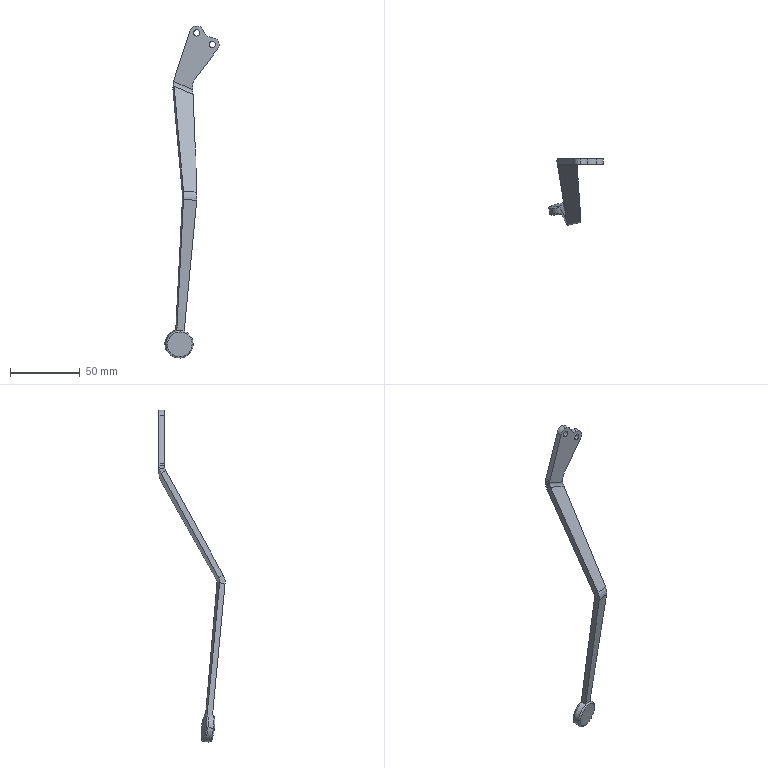Part | SolidWorks | features BaseBody 2 | 2 solids | 41 faces | box 39.153 x 47.602 x 238.853 mm | volume 12245 mm3 | cylinder 16 | plane 16 | spline 9 | commonest cylinder face diameters 20 x6 10 x3 4.454 x2 4.471 x2 12 x2 15.292 x1